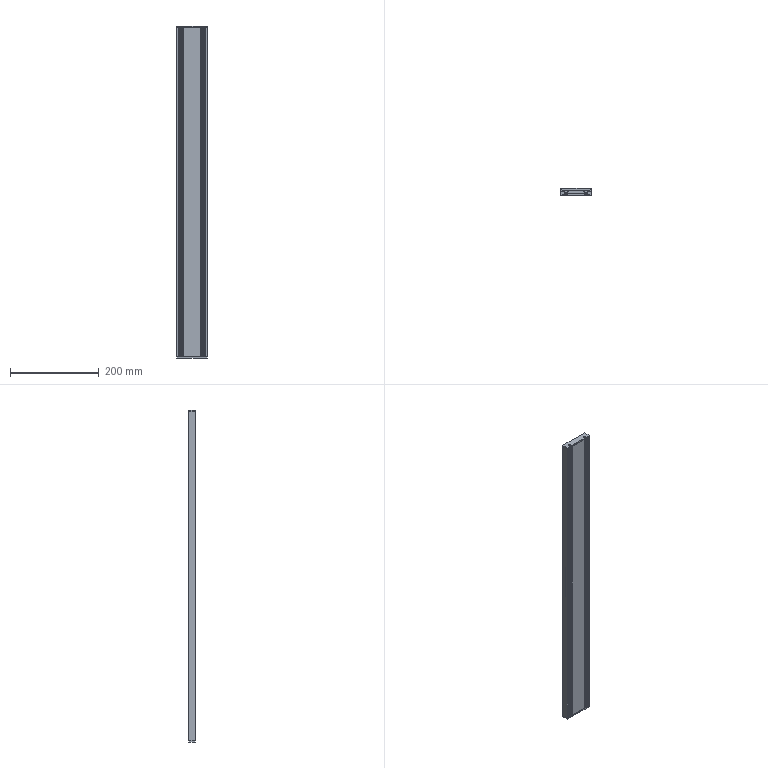Part | SolidWorks | features ICE 14, Fillet 3, Extrusion 1, MirrorSolid 1 | 4 solids | 1390 faces | box 70 x 15 x 750 mm | volume 474672 mm3 | plane 1340 | cylinder 50 | commonest cylinder face diameters 1 x12 2 x12 4 x8 6 x6 0.4 x4 1.1 x4